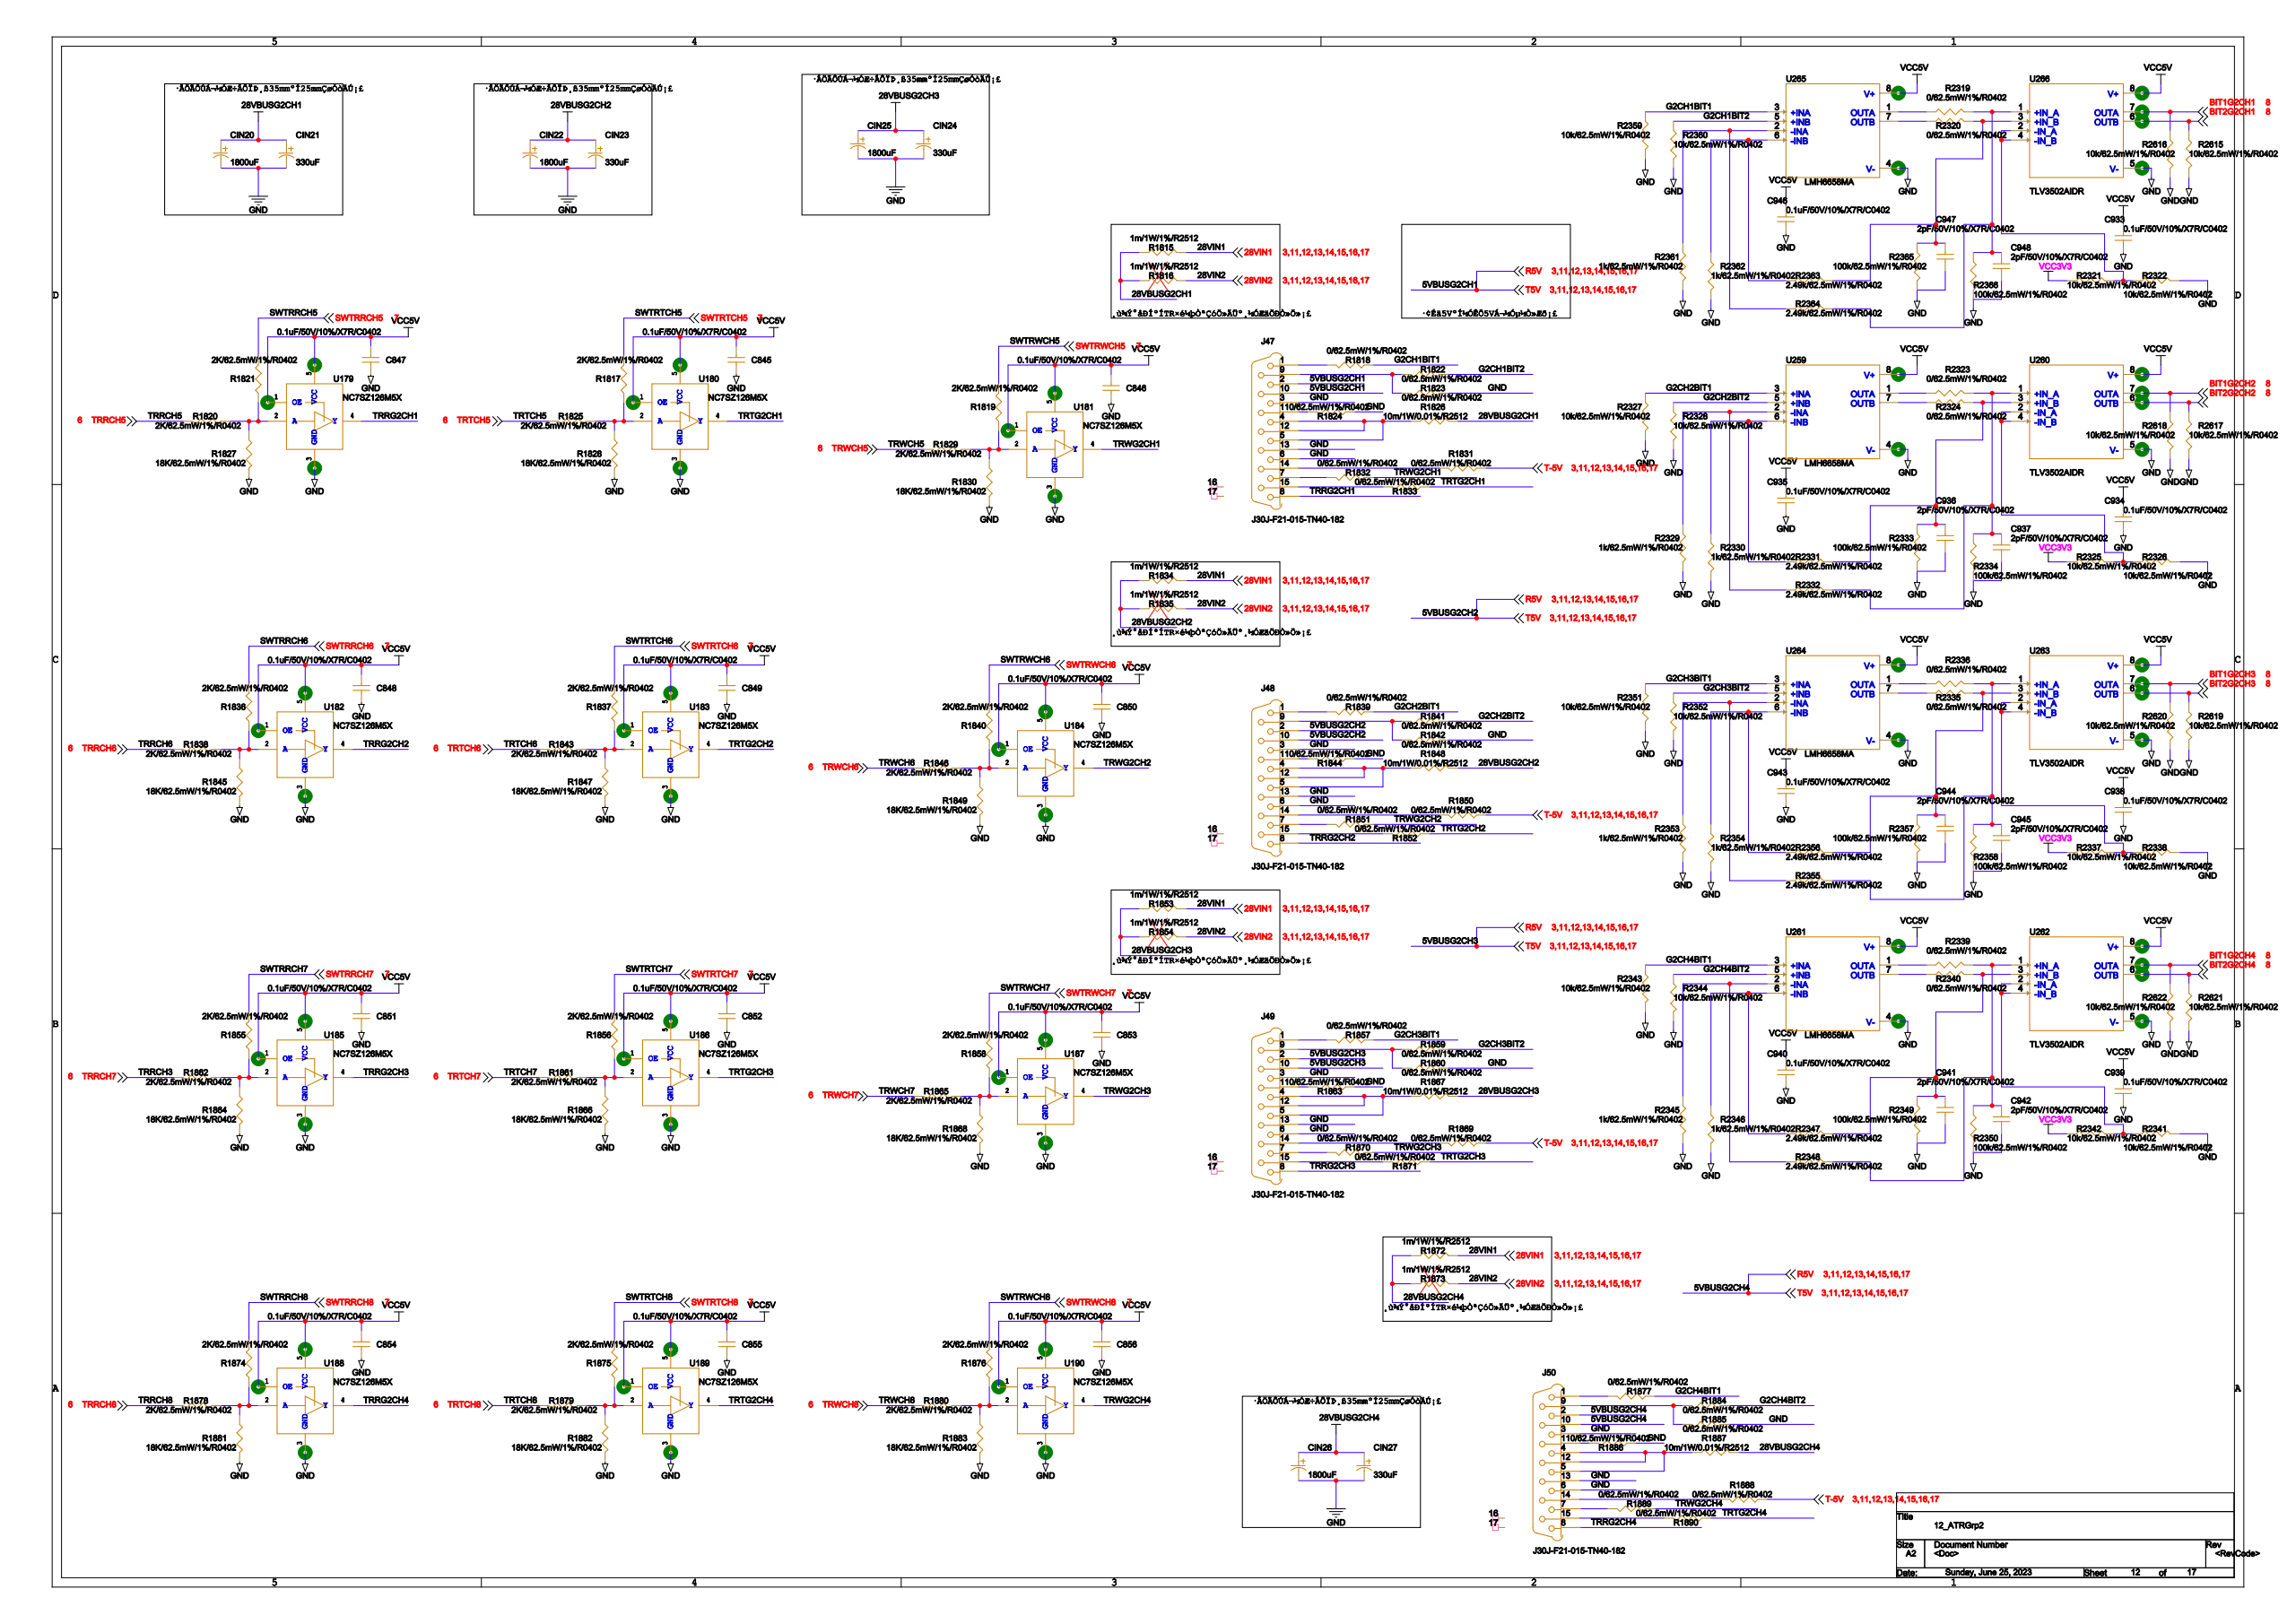Circuit board | Cadence Allegro | 2002 parts | 1538 nets | one sheet of the schematic
Parts on this sheet (reference | value | footprint):
C845 | 0.1uF/50V/10%/X7R/C0402 | 0402
C846 | 0.1uF/50V/10%/X7R/C0402 | 0402
C847 | 0.1uF/50V/10%/X7R/C0402 | 0402
C848 | 0.1uF/50V/10%/X7R/C0402 | 0402
C849 | 0.1uF/50V/10%/X7R/C0402 | 0402
C850 | 0.1uF/50V/10%/X7R/C0402 | 0402
C851 | 0.1uF/50V/10%/X7R/C0402 | 0402
C852 | 0.1uF/50V/10%/X7R/C0402 | 0402
C853 | 0.1uF/50V/10%/X7R/C0402 | 0402
C854 | 0.1uF/50V/10%/X7R/C0402 | 0402
C855 | 0.1uF/50V/10%/X7R/C0402 | 0402
C856 | 0.1uF/50V/10%/X7R/C0402 | 0402
C933 | 0.1uF/50V/10%/X7R/C0402 | 0402
C934 | 0.1uF/50V/10%/X7R/C0402 | 0402
C936 | 2pF/50V/10%/X7R/C0402 | 0402
C937 | 2pF/50V/10%/X7R/C0402 | 0402
C938 | 0.1uF/50V/10%/X7R/C0402 | 0402
C939 | 0.1uF/50V/10%/X7R/C0402 | 0402
C941 | 2pF/50V/10%/X7R/C0402 | 0402
C942 | 2pF/50V/10%/X7R/C0402 | 0402
C944 | 2pF/50V/10%/X7R/C0402 | 0402
C945 | 2pF/50V/10%/X7R/C0402 | 0402
C947 | 2pF/50V/10%/X7R/C0402 | 0402
C948 | 2pF/50V/10%/X7R/C0402 | 0402
CIN20 | ECF1HM182M27OTPO | AP-SMD_BD18-L27-W6_6-LS7_21
CIN21 | ECF1JM331G20OTPO | AP-SMD_BD10-L20-W6_6-LS7_21
CIN22 | ECF1HM182M27OTPO | AP-SMD_BD18-L27-W6_6-LS7_21
CIN23 | ECF1JM331G20OTPO | AP-SMD_BD10-L20-W6_6-LS7_21
CIN24 | ECF1JM331G20OTPO | AP-SMD_BD10-L20-W6_6-LS7_21
CIN25 | ECF1HM182M27OTPO | AP-SMD_BD18-L27-W6_6-LS7_21
CIN26 | ECF1HM182M27OTPO | AP-SMD_BD18-L27-W6_6-LS7_21
CIN27 | ECF1JM331G20OTPO | AP-SMD_BD10-L20-W6_6-LS7_21
J47 | J30J-F21-015-TN40-182 | J30J-F21-015-TN40-182
J48 | J30J-F21-015-TN40-182 | J30J-F21-015-TN40-182
J49 | J30J-F21-015-TN40-182 | J30J-F21-015-TN40-182
J50 | J30J-F21-015-TN40-182 | J30J-F21-015-TN40-182
R1815 | 1m/1W/1%/R2512 | 2512
R1816 | 1m/1W/1%/R2512 | 2512
R1817 | 2K/62.5mW/1%/R0402 | 0402
R1818 | 0/62.5mW/1%/R0402 | 0402
R1819 | 2K/62.5mW/1%/R0402 | 0402
R1820 | 2K/62.5mW/1%/R0402 | 0402
R1821 | 2K/62.5mW/1%/R0402 | 0402
R1822 | 0/62.5mW/1%/R0402 | 0402
R1823 | 0/62.5mW/1%/R0402 | 0402
R1824 | 0/62.5mW/1%/R0402 | 0402
R1825 | 2K/62.5mW/1%/R0402 | 0402
R1826 | 10m/1W/0.01%/R2512 | 2512
R1827 | 18K/62.5mW/1%/R0402 | 0402
R1828 | 18K/62.5mW/1%/R0402 | 0402
R1829 | 2K/62.5mW/1%/R0402 | 0402
R1830 | 18K/62.5mW/1%/R0402 | 0402
R1831 | 0/62.5mW/1%/R0402 | 0402
R1832 | 0/62.5mW/1%/R0402 | 0402
R1833 | 0/62.5mW/1%/R0402 | 0402
R1834 | 1m/1W/1%/R2512 | 2512
R1835 | 1m/1W/1%/R2512 | 2512
R1836 | 2K/62.5mW/1%/R0402 | 0402
R1837 | 2K/62.5mW/1%/R0402 | 0402
R1838 | 2K/62.5mW/1%/R0402 | 0402
R1839 | 0/62.5mW/1%/R0402 | 0402
R1840 | 2K/62.5mW/1%/R0402 | 0402
R1841 | 0/62.5mW/1%/R0402 | 0402
R1842 | 0/62.5mW/1%/R0402 | 0402
R1843 | 2K/62.5mW/1%/R0402 | 0402
R1844 | 0/62.5mW/1%/R0402 | 0402
R1845 | 18K/62.5mW/1%/R0402 | 0402
R1846 | 2K/62.5mW/1%/R0402 | 0402
R1847 | 18K/62.5mW/1%/R0402 | 0402
R1848 | 10m/1W/0.01%/R2512 | 2512
R1849 | 18K/62.5mW/1%/R0402 | 0402
R1850 | 0/62.5mW/1%/R0402 | 0402
R1851 | 0/62.5mW/1%/R0402 | 0402
R1852 | 0/62.5mW/1%/R0402 | 0402
R1853 | 1m/1W/1%/R2512 | 2512
R1854 | 1m/1W/1%/R2512 | 2512
R1855 | 2K/62.5mW/1%/R0402 | 0402
R1856 | 2K/62.5mW/1%/R0402 | 0402
R1857 | 0/62.5mW/1%/R0402 | 0402
R1858 | 2K/62.5mW/1%/R0402 | 0402
R1859 | 0/62.5mW/1%/R0402 | 0402
R1860 | 0/62.5mW/1%/R0402 | 0402
R1861 | 2K/62.5mW/1%/R0402 | 0402
R1862 | 2K/62.5mW/1%/R0402 | 0402
R1863 | 0/62.5mW/1%/R0402 | 0402
R1864 | 18K/62.5mW/1%/R0402 | 0402
R1865 | 2K/62.5mW/1%/R0402 | 0402
R1866 | 18K/62.5mW/1%/R0402 | 0402
R1867 | 10m/1W/0.01%/R2512 | 2512
R1868 | 18K/62.5mW/1%/R0402 | 0402
R1869 | 0/62.5mW/1%/R0402 | 0402
R1870 | 0/62.5mW/1%/R0402 | 0402
R1871 | 0/62.5mW/1%/R0402 | 0402
R1872 | 1m/1W/1%/R2512 | 2512
R1873 | 1m/1W/1%/R2512 | 2512
R1874 | 2K/62.5mW/1%/R0402 | 0402
R1875 | 2K/62.5mW/1%/R0402 | 0402
R1876 | 2K/62.5mW/1%/R0402 | 0402
R1877 | 0/62.5mW/1%/R0402 | 0402
R1878 | 2K/62.5mW/1%/R0402 | 0402
R1879 | 2K/62.5mW/1%/R0402 | 0402
R1880 | 2K/62.5mW/1%/R0402 | 0402
R1881 | 18K/62.5mW/1%/R0402 | 0402
R1882 | 18K/62.5mW/1%/R0402 | 0402
R1883 | 18K/62.5mW/1%/R0402 | 0402
R1884 | 0/62.5mW/1%/R0402 | 0402
R1885 | 0/62.5mW/1%/R0402 | 0402
R1886 | 0/62.5mW/1%/R0402 | 0402
R1887 | 10m/1W/0.01%/R2512 | 2512
R1888 | 0/62.5mW/1%/R0402 | 0402
R1889 | 0/62.5mW/1%/R0402 | 0402
R1890 | 0/62.5mW/1%/R0402 | 0402
R2319 | 0/62.5mW/1%/R0402 | 0402
R2320 | 0/62.5mW/1%/R0402 | 0402
R2321 | 10k/62.5mW/1%/R0402 | 0402
R2322 | 10k/62.5mW/1%/R0402 | 0402
R2323 | 0/62.5mW/1%/R0402 | 0402
R2324 | 0/62.5mW/1%/R0402 | 0402
R2325 | 10k/62.5mW/1%/R0402 | 0402
R2326 | 10k/62.5mW/1%/R0402 | 0402
R2327 | 10k/62.5mW/1%/R0402 | 0402
R2328 | 10k/62.5mW/1%/R0402 | 0402
R2329 | 1K/62.5mW/1%/R0402 | 0402
R2330 | 1K/62.5mW/1%/R0402 | 0402
R2332 | 2.49k/62.5mW/1%/R0402 | 0402
R2333 | 100k/62.5mW/1%/R0402 | 0402
R2334 | 100k/62.5mW/1%/R0402 | 0402
R2335 | 0/62.5mW/1%/R0402 | 0402
R2336 | 0/62.5mW/1%/R0402 | 0402
R2337 | 10k/62.5mW/1%/R0402 | 0402
R2338 | 10k/62.5mW/1%/R0402 | 0402
R2339 | 0/62.5mW/1%/R0402 | 0402
R2340 | 0/62.5mW/1%/R0402 | 0402
R2341 | 10k/62.5mW/1%/R0402 | 0402
R2342 | 10k/62.5mW/1%/R0402 | 0402
R2343 | 10k/62.5mW/1%/R0402 | 0402
R2344 | 10k/62.5mW/1%/R0402 | 0402
R2345 | 1K/62.5mW/1%/R0402 | 0402
R2346 | 1K/62.5mW/1%/R0402 | 0402
R2348 | 2.49k/62.5mW/1%/R0402 | 0402
R2349 | 100k/62.5mW/1%/R0402 | 0402
R2350 | 100k/62.5mW/1%/R0402 | 0402
R2351 | 10k/62.5mW/1%/R0402 | 0402
R2352 | 10k/62.5mW/1%/R0402 | 0402
R2353 | 1K/62.5mW/1%/R0402 | 0402
R2354 | 1K/62.5mW/1%/R0402 | 0402
R2355 | 2.49k/62.5mW/1%/R0402 | 0402
R2356 | 2.49k/62.5mW/1%/R0402 | 0402
R2357 | 100k/62.5mW/1%/R0402 | 0402
R2358 | 100k/62.5mW/1%/R0402 | 0402
R2359 | 10k/62.5mW/1%/R0402 | 0402
R2360 | 10k/62.5mW/1%/R0402 | 0402
R2361 | 1K/62.5mW/1%/R0402 | 0402
R2362 | 1K/62.5mW/1%/R0402 | 0402
R2364 | 2.49k/62.5mW/1%/R0402 | 0402
R2365 | 100k/62.5mW/1%/R0402 | 0402
R2366 | 100k/62.5mW/1%/R0402 | 0402
R2615 | 10k/62.5mW/1%/R0402 | 0402
R2616 | 10k/62.5mW/1%/R0402 | 0402
R2617 | 10k/62.5mW/1%/R0402 | 0402
R2618 | 10k/62.5mW/1%/R0402 | 0402
R2619 | 10k/62.5mW/1%/R0402 | 0402
R2620 | 10k/62.5mW/1%/R0402 | 0402
R2621 | 10k/62.5mW/1%/R0402 | 0402
R2622 | 10k/62.5mW/1%/R0402 | 0402
U179 | NC7SZ126M5X | SOT-23-5
U180 | NC7SZ126M5X | SOT-23-5
U181 | NC7SZ126M5X | SOT-23-5
U182 | NC7SZ126M5X | SOT-23-5
U183 | NC7SZ126M5X | SOT-23-5
U184 | NC7SZ126M5X | SOT-23-5
U185 | NC7SZ126M5X | SOT-23-5
U186 | NC7SZ126M5X | SOT-23-5
U187 | NC7SZ126M5X | SOT-23-5
U188 | NC7SZ126M5X | SOT-23-5
U189 | NC7SZ126M5X | SOT-23-5
U190 | NC7SZ126M5X | SOT-23-5
U259 | LMH6658MA | SOIC127P599X175-8N
U261 | LMH6658MA | SOIC127P599X175-8N
U263 | TLV3502AIDR | SOIC127P599X175-8N
U265 | LMH6658MA | SOIC127P599X175-8N
Nets of these parts (net: part-pin ...):
3.3V: R2321-1 R2325-1 R2337-1 R2342-1
AGND: C845-2 C846-2 C847-2 C848-2 C849-2 C850-2 C851-2 C852-2 C853-2 C854-2 C855-2 C856-2 C933-2 C934-2 C936-2 C937-2 C938-2 C939-2 C941-2 C942-2 C944-2 C945-2 C947-2 C948-2 CIN20-2 CIN21-2 CIN22-2 CIN23-2 CIN24-2 CIN25-2 CIN26-2 CIN27-2 J47-3 J47-6 J47-13 J48-3 J48-6 J48-13 J49-3 J49-6 J49-13 J50-3 J50-6 J50-13 R1823-1 R1824-1 R1827-1 R1828-1 R1830-1 R1842-1 R1844-1 R1845-1 R1847-1 R1849-1 R1860-1 R1863-1 R1864-1 R1866-1 R1868-1 R1881-1 R1882-1 R1883-1 R1885-1 R1886-1 R2322-2 R2326-2 R2327-2 R2328-2 R2329-2 R2330-2 R2333-2 R2334-2 R2338-2 R2341-2 R2343-2 R2344-2 R2345-2 R2346-2 R2349-2 R2350-2 R2351-2 R2352-2 R2353-2 R2354-2 R2357-2 R2358-2 R2359-2 R2360-2 R2361-2 R2362-2 R2365-2 R2366-2 R2615-2 R2616-2 R2617-2 R2618-2 R2619-2 R2620-2 R2621-2 R2622-2 U179-3 U180-3 U181-3 U182-3 U183-3 U184-3 U185-3 U186-3 U187-3 U188-3 U189-3 U190-3 U259-4 U261-4 U263-5 U265-4
VCC5V: C845-1 C846-1 C847-1 C848-1 C849-1 C850-1 C851-1 C852-1 C853-1 C854-1 C855-1 C856-1 C933-1 C934-1 C938-1 C939-1 U179-1 U179-5 U180-1 U180-5 U181-1 U181-5 U182-1 U182-5 U183-1 U183-5 U184-1 U184-5 U185-1 U185-5 U186-1 U186-5 U187-1 U187-5 U188-1 U188-5 U189-1 U189-5 U190-1 U190-5 U259-8 U261-8 U263-8 U265-8
28VIN1: R1815-2 R1816-2 R1834-2 R1835-2 R1853-2 R1854-2 R1872-2 R1873-2
R5V: J47-2 J47-10 J48-2 J48-10 J49-2 J49-10 J50-2 J50-10
T-5V: R1831-1 R1850-1 R1869-1 R1888-1
N24395982: R2330-1 U259-6
N24395992: C936-1 R2324-2 R2333-1
N24395970: R2329-1 R2332-1 U259-2
N24395990: C937-1 R2323-2 R2332-2 R2334-1
N24396536: R2346-1 U261-6
N24396546: C941-1 R2340-2 R2349-1
N24396524: R2345-1 R2348-1 U261-2
N24396544: C942-1 R2339-2 R2348-2 R2350-1
N24396348: R2353-1 R2355-1
N24396364: C945-1 R2336-2 R2355-2 R2358-1 U263-1
N24396352: R2354-1 R2356-1
N24396366: C944-1 R2335-2 R2356-2 R2357-1 U263-3
N24395802: R2362-1 U265-6
N24395812: C947-1 R2320-2 R2365-1
N24395798: R2361-1 R2364-1 U265-2
N24395810: C948-1 R2319-2 R2364-2 R2366-1
G2CH2BIT1: R1839-1 R2327-1 U259-3
G2CH2BIT2: R1841-1 R2328-1 U259-5
N24395986: R2323-1 U259-1
N24395988: R2324-1 U259-7
G2CH4BIT1: R1877-1 R2343-1 U261-3
G2CH4BIT2: R1884-1 R2344-1 U261-5
N24396540: R2339-1 U261-1
N24396542: R2340-1 U261-7
G2CH3BIT1: R1857-1 R2351-1
G2CH3BIT2: R1859-1 R2352-1
N24396360: R2336-1
N24396362: R2335-1
G2CH1BIT1: R1818-1 R2359-1 U265-3
G2CH1BIT2: R1822-1 R2360-1 U265-5
N24395806: R2319-1 U265-1
N24395808: R2320-1 U265-7
N24396044: R2325-2 R2326-1
BIT1G2CH2: R2618-1
BIT2G2CH2: R2617-1
N24396598: R2341-1 R2342-2
BIT1G2CH4: R2622-1
BIT2G2CH4: R2621-1
N24396418: R2337-2 R2338-1 U263-2 U263-4
BIT1G2CH3: R2620-1 U263-7
BIT2G2CH3: R2619-1 U263-6
N24395864: R2321-2 R2322-1
BIT1G2CH1: R2616-1
BIT2G2CH1: R2615-1
N23722815: J47-1 R1818-2
N23722828: J47-11 R1824-2
N23722830: J47-4 J47-5 J47-12 R1826-1
N23722842: J47-14 R1831-2
N23722846: J47-15 R1833-2
N23722844: J47-7 R1832-2
TRRG2CH1: J47-8 U179-4
N23722817: J47-9 R1822-2 R1823-2
N23723374: J48-1 R1839-2
N23723387: J48-11 R1844-2
N23723389: J48-4 J48-5 J48-12 R1848-1
N23723401: J48-14 R1850-2
N23723405: J48-15 R1852-2
N23723403: J48-7 R1851-2
TRRG2CH2: J48-8 U182-4
N23723376: J48-9 R1841-2 R1842-2
N23724001: J49-1 R1857-2
N23724014: J49-11 R1863-2
N23724016: J49-4 J49-5 J49-12 R1867-1
N23724028: J49-14 R1869-2
N23724032: J49-15 R1871-2
N23724030: J49-7 R1870-2
TRRG2CH3: J49-8 U185-4
N23724003: J49-9 R1859-2 R1860-2
N23724633: J50-1 R1877-2
N23724646: J50-11 R1886-2
N23724648: J50-4 J50-5 J50-12 R1887-1
N23724660: J50-14 R1888-2
N23724664: J50-15 R1890-2
N23724662: J50-7 R1889-2
TRRG2CH4: J50-8 U188-4
N23724635: J50-9 R1884-2 R1885-2
28VBUSG2CH1: CIN20-1 CIN21-1 R1815-1 R1816-1 R1826-2
28VBUSG2CH2: CIN22-1 CIN23-1 R1834-1 R1835-1 R1848-2
28VBUSG2CH3: CIN24-1 CIN25-1 R1853-1 R1854-1 R1867-2
28VBUSG2CH4: CIN26-1 CIN27-1 R1872-1 R1873-1 R1887-2
SWTRTCH5: R1817-1
N24002951: R1817-2 R1825-2 R1828-2 U180-2
SWTRWCH5: R1819-1
N24003439: R1819-2 R1829-2 R1830-2 U181-2
TRRCH5: R1820-1
N24003931: R1820-2 R1821-2 R1827-2 U179-2
SWTRRCH5: R1821-1
TRTCH5: R1825-1
TRWCH5: R1829-1
SWTRRCH6: R1836-1
N24004049: R1836-2 R1838-2 R1845-2 U182-2
SWTRTCH6: R1837-1
N24003069: R1837-2 R1843-2 R1847-2 U183-2
TRRCH6: R1838-1
SWTRWCH6: R1840-1
N24003561: R1840-2 R1846-2 R1849-2 U184-2
TRTCH6: R1843-1
TRWCH6: R1846-1
SWTRRCH7: R1855-1
N24004175: R1855-2 R1862-2 R1864-2 U185-2
SWTRTCH7: R1856-1
N24003195: R1856-2 R1861-2 R1866-2 U186-2
SWTRWCH7: R1858-1
N24003683: R1858-2 R1865-2 R1868-2 U187-2
TRTCH7: R1861-1
TRRCH7: R1862-1
TRWCH7: R1865-1
SWTRRCH8: R1874-1
N24004293: R1874-2 R1878-2 R1881-2 U188-2
SWTRTCH8: R1875-1
N24003317: R1875-2 R1879-2 R1882-2 U189-2
SWTRWCH8: R1876-1
N24003805: R1876-2 R1880-2 R1883-2 U190-2
TRRCH8: R1878-1
TRTCH8: R1879-1
TRWCH8: R1880-1
TRTG2CH1: R1833-1 U180-4
TRWG2CH1: R1832-1 U181-4
TRTG2CH2: R1852-1 U183-4
TRWG2CH2: R1851-1 U184-4
TRTG2CH3: R1871-1 U186-4
TRWG2CH3: R1870-1 U187-4
TRTG2CH4: R1890-1 U189-4
TRWG2CH4: R1889-1 U190-4